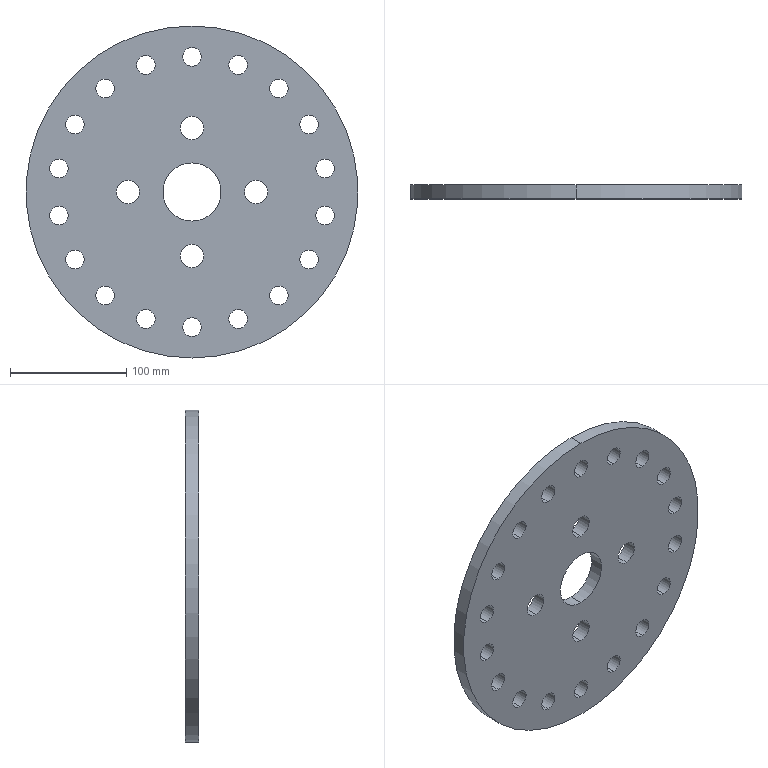Part | SolidWorks | features HoleWzd 2, Extrusion 1 | 1 solid | 50 faces | box 285 x 12 x 285 mm | volume 683457 mm3 | cylinder 48 | plane 2 | commonest cylinder face diameters 16 x36 20 x8 50 x2 285 x2